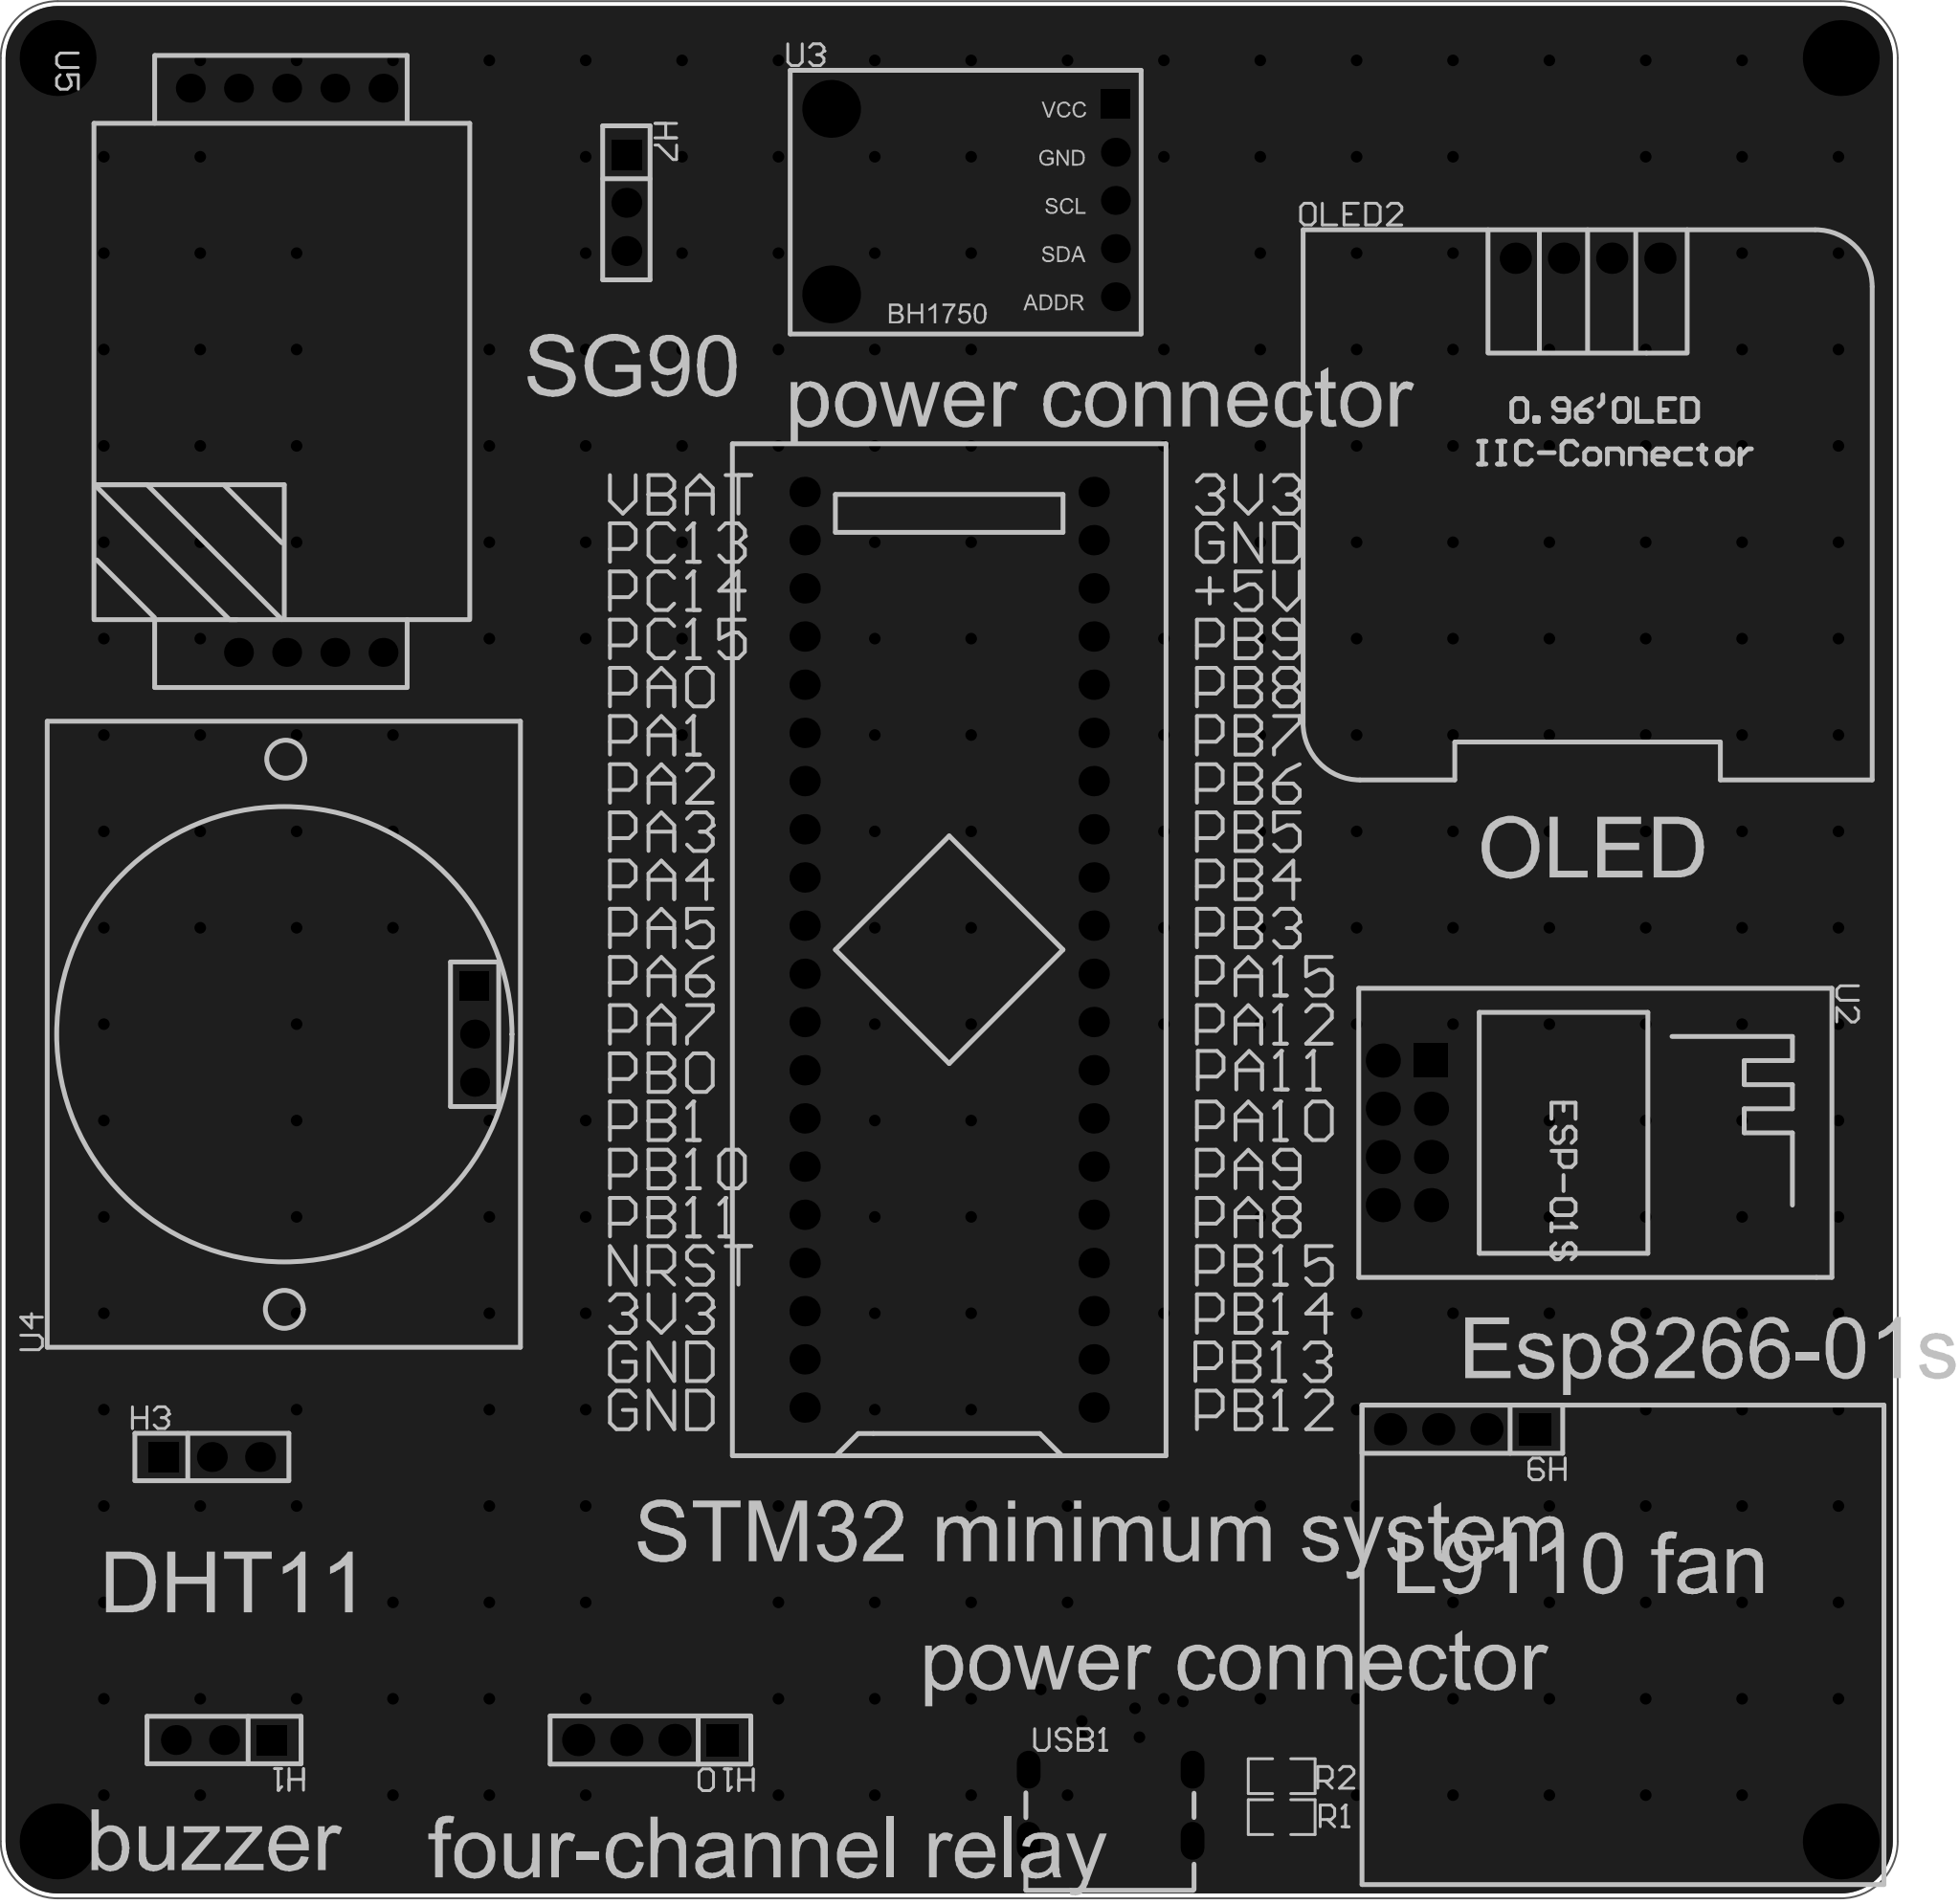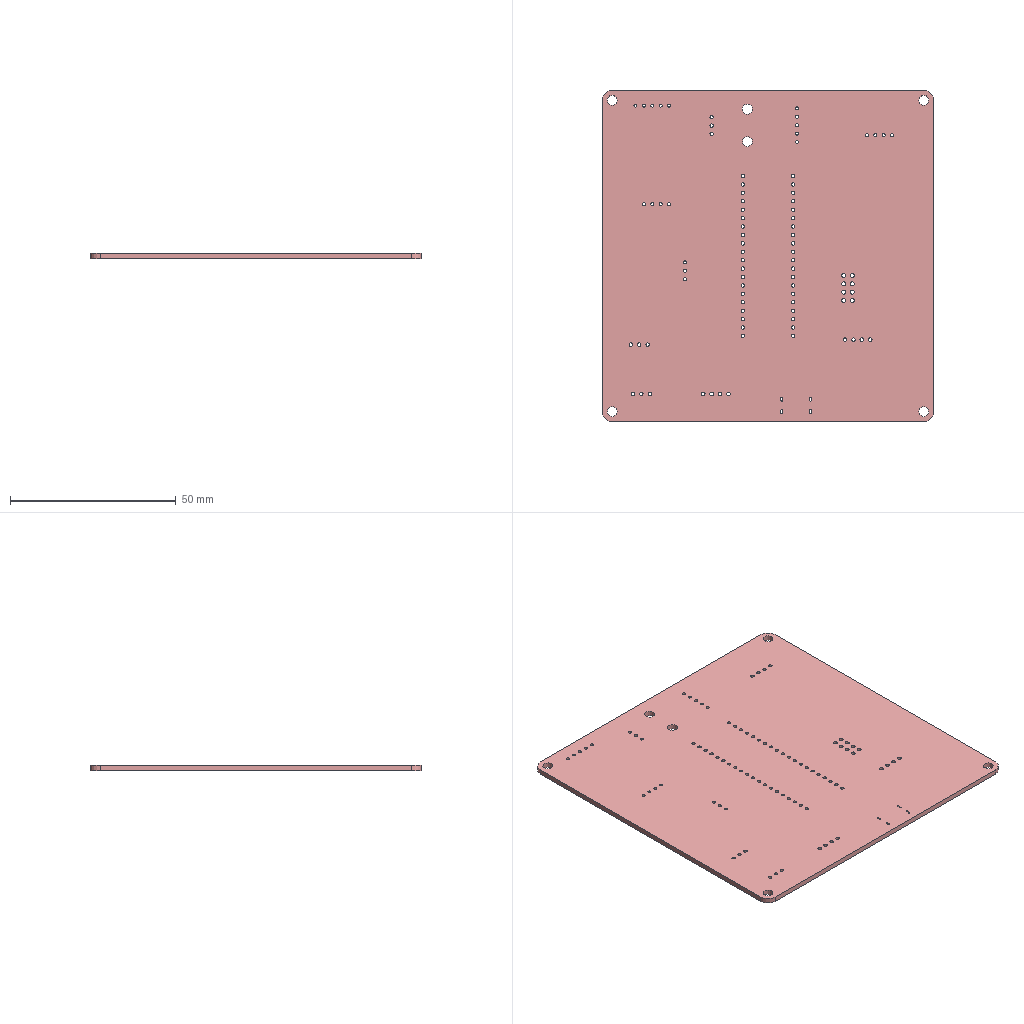Circuit board layout | Altium Designer | box 100 x 100 x 1.6 mm
Layer stack:
# Altium Designer layer stack of  (unit mm; dielectric type: 0 none, 1 core, 2 prepreg, 3 surface material)
index,name,kind,layer,copper_thickness_mm,dielectric_type,dielectric_thickness_mm,dielectric_material,dielectric_constant
0,Top Paste Mask Layer,other,,,,,,
1,Top Silkscreen Layer,other,,,,,,
2,Top Solder Mask Layer,dielectric,,,3,0.01,,3.3
3,Top Layer,copper,Top Layer,0.035,,,,
4,Dielectric1,dielectric,,,3,1.51,FR4,4.5
5,Bottom Layer,copper,Bottom Layer,0.035,,,,
6,Bottom Solder Mask Layer,dielectric,,,3,0.01,,3.3
7,Bottom Silkscreen Layer,other,,,,,,
8,Bottom Paste Mask Layer,other,,,,,,
# drill layer pairs: low layer,high layer
drill_pair,Top Layer,Bottom Layer
Part placement:
Designator,Comment,Layer,Footprint,Center-X(mm),Center-Y(mm),Rotation
U1,STM32F103C8T6-Card,TopLayer,CONN-TH_L53.3-W22.9_STM32F103C8T6-CARD,151.765,130.937,90
H1,,TopLayer,HDR-TH_3P-P2.54-V-F,113.538,89.281,180
H3,,TopLayer,HDR-TH_3P-P2.54-V-F,112.897,104.199,0
H7,,TopLayer,HDR-TH_3P-P2.54-V-F,134.747,170.307,270
H9,,TopLayer,HDR-TH_4P-P2.54-V-F,178.816,105.664,180
H10,,TopLayer,HDR-TH_4P-P2.54-V-F,136.017,89.281,180
OLED2,,TopLayer,0.96OLED_4P,185.42,167.386,0
U2,ESP-01S,TopLayer,WIFIM-TH_ESP-01S,175.895,121.285,270
U3,,TopLayer,BH1750光照传感器,153.035,170.434,0
U4,,TopLayer,HC-SR501_W32_H24,126.746,126.492,90
U5,,TopLayer,MH-Z19C-9PIN,116.84,161.481,270
USB1,,TopLayer,USB__TYPE-C-6P,160.274,86.106,0
R1,5.1K,TopLayer,R0805,169.291,85.217,0
R2,5.1K,TopLayer,R0805,169.291,87.376,0
Pad and via stacks:
# Altium Designer via and pad stacks of  (unit mm). Each distinct definition once, with the count of objects using it.
# via: kind,start_layer,end_layer,hole_mm,diameter_mm,mode(0 simple;1 top-mid-bottom;2 full stack),diameter_per_layer,count,example_net
# pad: kind,layer,hole_mm,hole_type(0 round;1 square;2 slot),plating,top_size,top_shape(1 round;2 rect;3 octagon;9 rounded rect),mid_size,bottom_size,mode,footprint,size_per_layer,count,example
pad,Multi-Layer,3,0,plated,4x4,1,4x4,4x4,0,,,4,1
pad,Multi-Layer,1,0,plated,1.6x1.6,1,1.6x1.6,1.6x1.6,0,CONN-TH_L53.3-W22.9_STM32F103C8T6-CARD,,40,U1.1
pad,Multi-Layer,1.02,0,plated,1.575x1.575,1,1.575x1.575,1.575x1.575,0,HDR-TH_3P-P2.54-V-F,,6,H1.3
pad,Multi-Layer,1.02,0,plated,1.575x1.575,2,1.575x1.575,1.575x1.575,0,HDR-TH_3P-P2.54-V-F,,3,H1.1
pad,Multi-Layer,1.1,0,plated,1.7x1.7,2,1.7x1.7,1.7x1.7,0,HDR-TH_4P-P2.54-V-F,,2,H9.1
pad,Multi-Layer,1.1,0,plated,1.7x1.7,1,1.7x1.7,1.7x1.7,0,HDR-TH_4P-P2.54-V-F,,6,H9.2
pad,Multi-Layer,1,0,plated,1.65x1.65,1,1.65x1.65,1.65x1.65,0,0.96OLED_4P,,4,OLED2.4
pad,Multi-Layer,1.2,0,plated,1.8x1.8,2,1.8x1.8,1.8x1.8,0,WIFIM-TH_ESP-01S,,1,U2.1
pad,Multi-Layer,1.2,0,plated,1.8x1.8,1,1.8x1.8,1.8x1.8,0,WIFIM-TH_ESP-01S,,7,U2.2
pad,Multi-Layer,3.048,0,unplated,3.048x3.048,1,3.048x3.048,3.048x3.048,0,BH1750\u00B9\u00E2\u00D5\u00D5\u00B4\u00AB\u00B8\u00D0\u00C6\u00F7,,2,U3.
pad,Multi-Layer,0.9144,0,plated,1.524x1.524,2,1.524x1.524,1.524x1.524,0,BH1750\u00B9\u00E2\u00D5\u00D5\u00B4\u00AB\u00B8\u00D0\u00C6\u00F7,,1,U3.1
pad,Multi-Layer,0.9144,0,plated,1.524x1.524,1,1.524x1.524,1.524x1.524,0,BH1750\u00B9\u00E2\u00D5\u00D5\u00B4\u00AB\u00B8\u00D0\u00C6\u00F7,,4,U3.4
pad,Multi-Layer,0.9144,0,plated,1.524x1.524,2,1.524x1.524,1.524x1.524,0,HC-SR501_W32_H24,,1,U4.1
pad,Multi-Layer,0.9144,0,plated,1.524x1.524,1,1.524x1.524,1.524x1.524,0,HC-SR501_W32_H24,,2,U4.2
pad,Multi-Layer,0.9144,0,plated,1.524x1.524,1,1.524x1.524,1.524x1.524,0,MH-Z19C-9PIN,,9,U5.9
pad,Multi-Layer,0.6,2,plated,1.25x2,1,1.25x2,1.25x2,0,USB_ TYPE-C-6P,,4,USB1.8
pad,Top Layer,0,0,plated,0.7x1.2,2,0.7x1.2,0.7x1.2,0,USB_ TYPE-C-6P,,2,USB1.A5
pad,Top Layer,0,0,plated,0.8x1.2,2,0.8x1.2,0.8x1.2,0,USB_ TYPE-C-6P,,2,USB1.B9
pad,Top Layer,0,0,plated,0.9x1.2,2,0.9x1.2,0.9x1.2,0,USB_ TYPE-C-6P,,2,USB1.B12
pad,Top Layer,0,0,plated,1.133x1.377,2,1.133x1.377,1.133x1.377,0,R0805,,4,R1.2
via,Top Layer,Bottom Layer,0.3048,0.61,0,,273,+5V
Copper pours:
name,layer,net,type(0 solid;1 hatched;2 none)
Bottom Layer-GND,Bottom Layer,GND,0
Top Layer-GND,Top Layer,GND,0
Design rules, without the lines most boards share:
# Altium Designer design rules of  (exported by Altium Designer, unit mm)
# columns: name | kind | enabled | priority | scope1 | scope2 | descriptor | typed fields (field=value)
Copper_copperRegion_copperThickness1oz | 0 | disabled | 4 | All | All | Clearance Constraint (Gap=5.984mil) (Disabled)(All),(All) | gap=0.152
Copper_copperRegion_copperThickness1oz_1 | 63 | disabled | 4 | All | All | Board Clearance Constraint (Gap=0mil) (Disabled)(All) |
Copper_copperRegion_Copper_copperRegion | 0 | disabled | 5 | All | All | Clearance Constraint (Gap=5.984mil) (Disabled)(All),(All) | gap=0.152
Copper_copperRegion_Copper_copperRegion_1 | 63 | disabled | 5 | All | All | Board Clearance Constraint (Gap=0mil) (Disabled)(All) |
copperThickness1oz | 0 | enabled | 6 | All | All | Clearance Constraint (Gap=5.984mil) (All),(All) | gap=0.152
copperThickness1oz_1 | 63 | enabled | 6 | All | All | Board Clearance Constraint (Gap=0mil) (All) |
copperRegion_copperThickness1oz | 20 | disabled | 1 | All | All | Polygon Connect Rule(Relief Connect )(Conductor Width=10mil) (Relief Angle=90 Angle) (Entries=4) (Air Gap Width=10mil) (Disabled)(All),(All) | connect_style(0=relief,1=direct,2=none)=0 relief_conductor_width=0.254 relief_entries=4
copperRegion_Copper_copperRegion | 20 | disabled | 2 | All | All | Polygon Connect Rule(Relief Connect )(Conductor Width=10mil) (Relief Angle=90 Angle) (Entries=4) (Air Gap Width=10mil) (Disabled)(All),(All) | connect_style(0=relief,1=direct,2=none)=0 relief_conductor_width=0.254 relief_entries=4
copperRegion | 20 | enabled | 3 | All | All | Polygon Connect Rule(Relief Connect )(Conductor Width=10mil) (Relief Angle=90 Angle) (Entries=4) (Air Gap Width=10mil) (All),(All) | connect_style(0=relief,1=direct,2=none)=0 relief_conductor_width=0.254 relief_entries=4